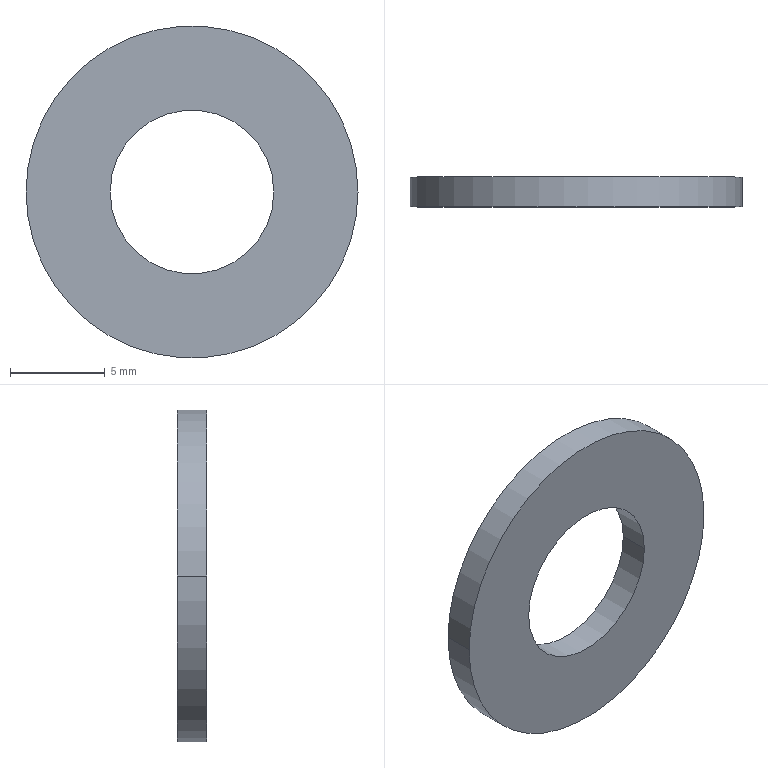Part | NX | features BREP 1 | 1 solid | 6 faces | box 17.526 x 1.575 x 17.526 mm | volume 287.666 mm3 | cylinder 4 | plane 2 | commonest cylinder face diameters 8.636 x2 17.526 x2
STEP:
#1=CARTESIAN_POINT('',(-8.763,0.,0.));
#2=VERTEX_POINT('',#1);
#3=CARTESIAN_POINT('',(8.763,0.,0.));
#4=VERTEX_POINT('',#3);
#5=CARTESIAN_POINT('',(0.,0.,0.));
#6=DIRECTION('',(0.,1.,0.));
#7=DIRECTION('',(-1.,0.,0.));
#8=AXIS2_PLACEMENT_3D('',#5,#6,#7);
#9=CIRCLE('',#8,8.763);
#10=EDGE_CURVE('',#2,#4,#9,.T.);
#11=ORIENTED_EDGE('',*,*,#10,.F.);
#12=CARTESIAN_POINT('',(0.,0.,0.));
#13=DIRECTION('',(0.,1.,0.));
#14=DIRECTION('',(1.,0.,0.));
#15=AXIS2_PLACEMENT_3D('',#12,#13,#14);
#16=CIRCLE('',#15,8.763);
#17=EDGE_CURVE('',#4,#2,#16,.T.);
#18=ORIENTED_EDGE('',*,*,#17,.F.);
#19=EDGE_LOOP('',(#11,#18));
#20=FACE_BOUND('',#19,.T.);
#21=CARTESIAN_POINT('',(-4.318,0.,0.));
#22=VERTEX_POINT('',#21);
#23=CARTESIAN_POINT('',(4.318,0.,0.));
#24=VERTEX_POINT('',#23);
#25=CARTESIAN_POINT('',(0.,0.,0.));
#26=DIRECTION('',(0.,-1.,0.));
#27=DIRECTION('',(-1.,0.,0.));
#28=AXIS2_PLACEMENT_3D('',#25,#26,#27);
#29=CIRCLE('',#28,4.318);
#30=EDGE_CURVE('',#22,#24,#29,.T.);
#31=ORIENTED_EDGE('',*,*,#30,.F.);
#32=CARTESIAN_POINT('',(0.,0.,0.));
#33=DIRECTION('',(0.,-1.,0.));
#34=DIRECTION('',(1.,0.,0.));
#35=AXIS2_PLACEMENT_3D('',#32,#33,#34);
#36=CIRCLE('',#35,4.318);
#37=EDGE_CURVE('',#24,#22,#36,.T.);
#38=ORIENTED_EDGE('',*,*,#37,.F.);
#39=EDGE_LOOP('',(#31,#38));
#40=FACE_BOUND('',#39,.T.);
#41=CARTESIAN_POINT('',(0.,0.,0.));
#42=DIRECTION('',(0.,1.,0.));
#43=DIRECTION('',(1.,0.,0.));
#44=AXIS2_PLACEMENT_3D('',#41,#42,#43);
#45=PLANE('',#44);
#46=ADVANCED_FACE('',(#20,#40),#45,.F.);
#47=CARTESIAN_POINT('',(-8.763,1.575,0.));
#48=VERTEX_POINT('',#47);
#49=CARTESIAN_POINT('',(-8.763,0.,0.));
#50=DIRECTION('',(0.,1.,0.));
#51=VECTOR('',#50,1000.);
#52=LINE('',#49,#51);
#53=EDGE_CURVE('',#2,#48,#52,.T.);
#54=ORIENTED_EDGE('',*,*,#53,.T.);
#55=CARTESIAN_POINT('',(8.763,1.575,0.));
#56=VERTEX_POINT('',#55);
#57=CARTESIAN_POINT('',(0.,1.575,0.));
#58=DIRECTION('',(0.,1.,0.));
#59=DIRECTION('',(1.,0.,0.));
#60=AXIS2_PLACEMENT_3D('',#57,#58,#59);
#61=CIRCLE('',#60,8.763);
#62=EDGE_CURVE('',#56,#48,#61,.T.);
#63=ORIENTED_EDGE('',*,*,#62,.F.);
#64=CARTESIAN_POINT('',(8.763,0.,0.));
#65=DIRECTION('',(0.,1.,0.));
#66=VECTOR('',#65,1000.);
#67=LINE('',#64,#66);
#68=EDGE_CURVE('',#4,#56,#67,.T.);
#69=ORIENTED_EDGE('',*,*,#68,.F.);
#70=ORIENTED_EDGE('',*,*,#17,.T.);
#71=EDGE_LOOP('',(#54,#63,#69,#70));
#72=FACE_BOUND('',#71,.T.);
#73=CARTESIAN_POINT('',(0.,0.,0.));
#74=DIRECTION('',(0.,1.,0.));
#75=DIRECTION('',(1.,0.,0.));
#76=AXIS2_PLACEMENT_3D('',#73,#74,#75);
#77=CYLINDRICAL_SURFACE('',#76,8.763);
#78=ADVANCED_FACE('',(#72),#77,.T.);
#79=ORIENTED_EDGE('',*,*,#68,.T.);
#80=CARTESIAN_POINT('',(0.,1.575,0.));
#81=DIRECTION('',(0.,1.,0.));
#82=DIRECTION('',(-1.,0.,0.));
#83=AXIS2_PLACEMENT_3D('',#80,#81,#82);
#84=CIRCLE('',#83,8.763);
#85=EDGE_CURVE('',#48,#56,#84,.T.);
#86=ORIENTED_EDGE('',*,*,#85,.F.);
#87=ORIENTED_EDGE('',*,*,#53,.F.);
#88=ORIENTED_EDGE('',*,*,#10,.T.);
#89=EDGE_LOOP('',(#79,#86,#87,#88));
#90=FACE_BOUND('',#89,.T.);
#91=CARTESIAN_POINT('',(0.,0.,0.));
#92=DIRECTION('',(0.,1.,0.));
#93=DIRECTION('',(1.,0.,0.));
#94=AXIS2_PLACEMENT_3D('',#91,#92,#93);
#95=CYLINDRICAL_SURFACE('',#94,8.763);
#96=ADVANCED_FACE('',(#90),#95,.T.);
#97=ORIENTED_EDGE('',*,*,#85,.T.);
#98=ORIENTED_EDGE('',*,*,#62,.T.);
#99=EDGE_LOOP('',(#97,#98));
#100=FACE_BOUND('',#99,.T.);
#101=CARTESIAN_POINT('',(-4.318,1.575,0.));
#102=VERTEX_POINT('',#101);
#103=CARTESIAN_POINT('',(4.318,1.575,0.));
#104=VERTEX_POINT('',#103);
#105=CARTESIAN_POINT('',(0.,1.575,0.));
#106=DIRECTION('',(0.,-1.,0.));
#107=DIRECTION('',(-1.,0.,0.));
#108=AXIS2_PLACEMENT_3D('',#105,#106,#107);
#109=CIRCLE('',#108,4.318);
#110=EDGE_CURVE('',#102,#104,#109,.T.);
#111=ORIENTED_EDGE('',*,*,#110,.T.);
#112=CARTESIAN_POINT('',(0.,1.575,0.));
#113=DIRECTION('',(0.,-1.,0.));
#114=DIRECTION('',(1.,0.,0.));
#115=AXIS2_PLACEMENT_3D('',#112,#113,#114);
#116=CIRCLE('',#115,4.318);
#117=EDGE_CURVE('',#104,#102,#116,.T.);
#118=ORIENTED_EDGE('',*,*,#117,.T.);
#119=EDGE_LOOP('',(#111,#118));
#120=FACE_BOUND('',#119,.T.);
#121=CARTESIAN_POINT('',(0.,1.575,0.));
#122=DIRECTION('',(0.,1.,0.));
#123=DIRECTION('',(1.,0.,0.));
#124=AXIS2_PLACEMENT_3D('',#121,#122,#123);
#125=PLANE('',#124);
#126=ADVANCED_FACE('',(#100,#120),#125,.T.);
#127=CARTESIAN_POINT('',(-4.318,0.,0.));
#128=DIRECTION('',(0.,1.,0.));
#129=VECTOR('',#128,1000.);
#130=LINE('',#127,#129);
#131=EDGE_CURVE('',#22,#102,#130,.T.);
#132=ORIENTED_EDGE('',*,*,#131,.T.);
#133=ORIENTED_EDGE('',*,*,#117,.F.);
#134=CARTESIAN_POINT('',(4.318,0.,0.));
#135=DIRECTION('',(0.,1.,0.));
#136=VECTOR('',#135,1000.);
#137=LINE('',#134,#136);
#138=EDGE_CURVE('',#24,#104,#137,.T.);
#139=ORIENTED_EDGE('',*,*,#138,.F.);
#140=ORIENTED_EDGE('',*,*,#37,.T.);
#141=EDGE_LOOP('',(#132,#133,#139,#140));
#142=FACE_BOUND('',#141,.T.);
#143=CARTESIAN_POINT('',(0.,0.,0.));
#144=DIRECTION('',(0.,1.,0.));
#145=DIRECTION('',(1.,0.,0.));
#146=AXIS2_PLACEMENT_3D('',#143,#144,#145);
#147=CYLINDRICAL_SURFACE('',#146,4.318);
#148=ADVANCED_FACE('',(#142),#147,.F.);
#149=ORIENTED_EDGE('',*,*,#138,.T.);
#150=ORIENTED_EDGE('',*,*,#110,.F.);
#151=ORIENTED_EDGE('',*,*,#131,.F.);
#152=ORIENTED_EDGE('',*,*,#30,.T.);
#153=EDGE_LOOP('',(#149,#150,#151,#152));
#154=FACE_BOUND('',#153,.T.);
#155=CARTESIAN_POINT('',(0.,0.,0.));
#156=DIRECTION('',(0.,1.,0.));
#157=DIRECTION('',(1.,0.,0.));
#158=AXIS2_PLACEMENT_3D('',#155,#156,#157);
#159=CYLINDRICAL_SURFACE('',#158,4.318);
#160=ADVANCED_FACE('',(#154),#159,.F.);
#161=CLOSED_SHELL('',(#46,#78,#96,#126,#148,#160));
#162=MANIFOLD_SOLID_BREP('',#161);
#163=(LENGTH_UNIT()NAMED_UNIT(*)SI_UNIT(.MILLI.,.METRE.));
#164=UNCERTAINTY_MEASURE_WITH_UNIT(LENGTH_MEASURE(0.00001),#163,'','');
#165=(NAMED_UNIT(*)PLANE_ANGLE_UNIT()SI_UNIT($,.RADIAN.));
#166=(NAMED_UNIT(*)SI_UNIT($,.STERADIAN.)SOLID_ANGLE_UNIT());
#167=(GEOMETRIC_REPRESENTATION_CONTEXT(3)GLOBAL_UNCERTAINTY_ASSIGNED_CONTEXT((#164))GLOBAL_UNIT_ASSIGNED_CONTEXT((#163,#165,#166))REPRESENTATION_CONTEXT('',''));
#168=ADVANCED_BREP_SHAPE_REPRESENTATION('',(#162),#167);